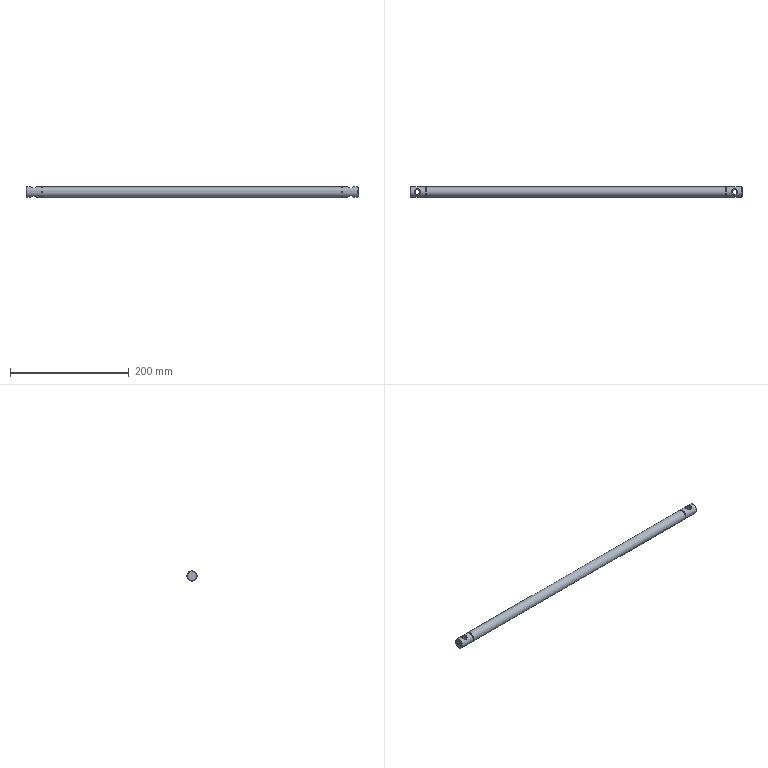Part | STEP file | 7100803 | 1 solid | 19 faces | box 560 x 17 x 17 mm | volume 125657 mm3 | cylinder 7 | plane 6 | spline 4 | cone 2 | commonest cylinder face diameters 17 x3 8 x2 15.6 x2